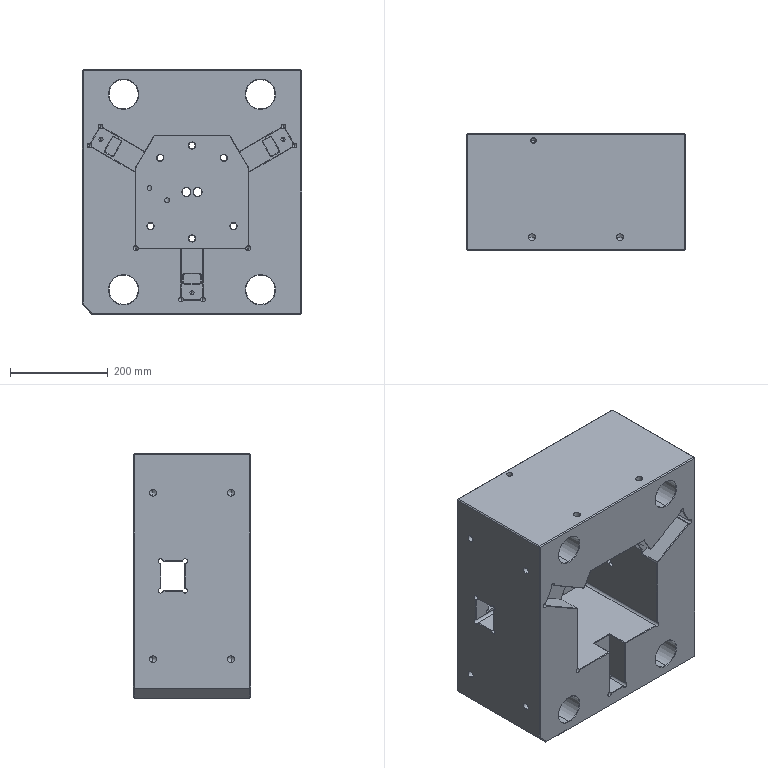Part | STEP file | P1 - 1 cav | 1 solid | 515 faces | box 450 x 240 x 500 mm | volume 38190234 mm3 | cylinder 184 | plane 167 | cone 164 | commonest cylinder face diameters 10 x40 14 x40 8 x24 34 x16 6 x14 13 x12